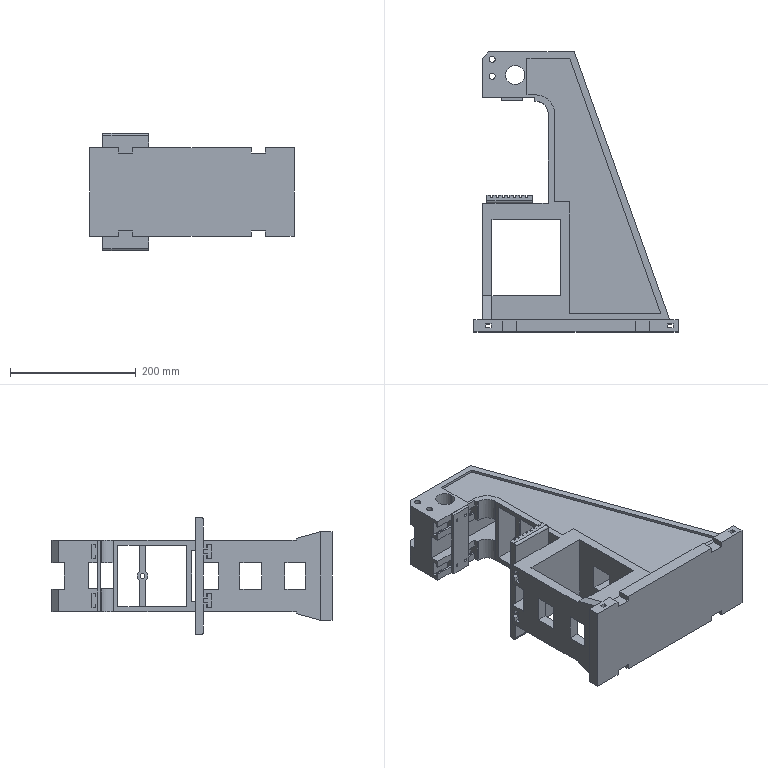Part | SolidWorks | features Cut 13, ICE 7, MoveFace 2, Chamfer 1, Extrusion 1, Fillet 1, MirrorPattern 1 | 6 solids | 271 faces | box 324.62 x 445 x 186.175 mm | volume 5513509 mm3 | plane 238 | cylinder 33 | commonest cylinder face diameters 4 x16 9.805 x6 7.484 x2 8 x2 16.309 x2 30.343 x2